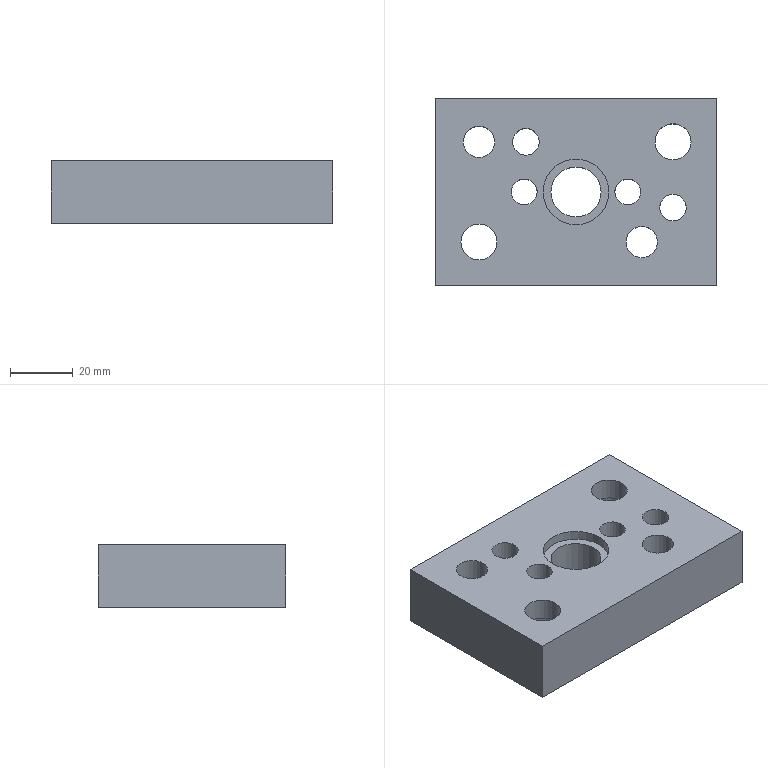Part | STEP file | lll_id3314_x_t | 1 solid | 21 faces | box 90 x 60 x 20 mm | volume 87938 mm3 | cylinder 12 | plane 9 | commonest cylinder face diameters 8.2 x2 8.505 x2 10 x2 11.509 x2 18.007 x2 16 x1
STEP:
#1=CARTESIAN_POINT('',(1798.,-16.,2.5));
#2=VERTEX_POINT('',#1);
#3=CARTESIAN_POINT('',(1803.,-16.,2.5));
#4=DIRECTION('',(0.,0.,-1.));
#5=DIRECTION('',(-1.,0.,0.));
#6=AXIS2_PLACEMENT_3D('',#3,#4,#5);
#7=CIRCLE('',#6,5.);
#8=EDGE_CURVE('',#2,#2,#7,.T.);
#9=ORIENTED_EDGE('',*,*,#8,.F.);
#10=EDGE_LOOP('',(#9));
#11=FACE_BOUND('',#10,.T.);
#12=CARTESIAN_POINT('',(1746.,16.,2.5));
#13=VERTEX_POINT('',#12);
#14=CARTESIAN_POINT('',(1751.,16.,2.5));
#15=DIRECTION('',(0.,0.,-1.));
#16=DIRECTION('',(-1.,0.,0.));
#17=AXIS2_PLACEMENT_3D('',#14,#15,#16);
#18=CIRCLE('',#17,5.);
#19=EDGE_CURVE('',#13,#13,#18,.T.);
#20=ORIENTED_EDGE('',*,*,#19,.F.);
#21=EDGE_LOOP('',(#20));
#22=FACE_BOUND('',#21,.T.);
#23=CARTESIAN_POINT('',(1813.,-9.253,2.5));
#24=VERTEX_POINT('',#23);
#25=CARTESIAN_POINT('',(1813.,-5.,2.5));
#26=DIRECTION('',(0.,0.,1.));
#27=DIRECTION('',(0.,-1.,0.));
#28=AXIS2_PLACEMENT_3D('',#25,#26,#27);
#29=CIRCLE('',#28,4.253);
#30=EDGE_CURVE('',#24,#24,#29,.T.);
#31=ORIENTED_EDGE('',*,*,#30,.T.);
#32=EDGE_LOOP('',(#31));
#33=FACE_BOUND('',#32,.T.);
#34=CARTESIAN_POINT('',(1741.996,-16.,2.5));
#35=VERTEX_POINT('',#34);
#36=CARTESIAN_POINT('',(1751.,-16.,2.5));
#37=DIRECTION('',(0.,0.,1.));
#38=DIRECTION('',(-1.,0.,0.));
#39=AXIS2_PLACEMENT_3D('',#36,#37,#38);
#40=CIRCLE('',#39,9.004);
#41=EDGE_CURVE('',#35,#35,#40,.T.);
#42=ORIENTED_EDGE('',*,*,#41,.T.);
#43=EDGE_LOOP('',(#42));
#44=FACE_BOUND('',#43,.T.);
#45=CARTESIAN_POINT('',(1827.,-30.,2.5));
#46=VERTEX_POINT('',#45);
#47=CARTESIAN_POINT('',(1827.,30.,2.5));
#48=VERTEX_POINT('',#47);
#49=CARTESIAN_POINT('',(1827.,0.,2.5));
#50=DIRECTION('',(0.,1.,0.));
#51=VECTOR('',#50,1.);
#52=LINE('',#49,#51);
#53=EDGE_CURVE('',#46,#48,#52,.T.);
#54=ORIENTED_EDGE('',*,*,#53,.F.);
#55=CARTESIAN_POINT('',(1737.,-30.,2.5));
#56=VERTEX_POINT('',#55);
#57=CARTESIAN_POINT('',(1782.,-30.,2.5));
#58=DIRECTION('',(1.,0.,0.));
#59=VECTOR('',#58,1.);
#60=LINE('',#57,#59);
#61=EDGE_CURVE('',#56,#46,#60,.T.);
#62=ORIENTED_EDGE('',*,*,#61,.F.);
#63=CARTESIAN_POINT('',(1737.,30.,2.5));
#64=VERTEX_POINT('',#63);
#65=CARTESIAN_POINT('',(1737.,0.,2.5));
#66=DIRECTION('',(0.,-1.,0.));
#67=VECTOR('',#66,1.);
#68=LINE('',#65,#67);
#69=EDGE_CURVE('',#64,#56,#68,.T.);
#70=ORIENTED_EDGE('',*,*,#69,.F.);
#71=CARTESIAN_POINT('',(1782.,30.,2.5));
#72=DIRECTION('',(-1.,0.,0.));
#73=VECTOR('',#72,1.);
#74=LINE('',#71,#73);
#75=EDGE_CURVE('',#48,#64,#74,.T.);
#76=ORIENTED_EDGE('',*,*,#75,.F.);
#77=EDGE_LOOP('',(#54,#62,#70,#76));
#78=FACE_BOUND('',#77,.T.);
#79=CARTESIAN_POINT('',(1803.997,16.,2.5));
#80=VERTEX_POINT('',#79);
#81=CARTESIAN_POINT('',(1813.,16.,2.5));
#82=DIRECTION('',(0.,0.,1.));
#83=DIRECTION('',(-1.,0.,0.));
#84=AXIS2_PLACEMENT_3D('',#81,#82,#83);
#85=CIRCLE('',#84,9.004);
#86=EDGE_CURVE('',#80,#80,#85,.T.);
#87=ORIENTED_EDGE('',*,*,#86,.T.);
#88=EDGE_LOOP('',(#87));
#89=FACE_BOUND('',#88,.T.);
#90=CARTESIAN_POINT('',(1761.4,0.,2.5));
#91=VERTEX_POINT('',#90);
#92=CARTESIAN_POINT('',(1765.5,0.,2.5));
#93=DIRECTION('',(0.,0.,-1.));
#94=DIRECTION('',(-1.,0.,0.));
#95=AXIS2_PLACEMENT_3D('',#92,#93,#94);
#96=CIRCLE('',#95,4.1);
#97=EDGE_CURVE('',#91,#91,#96,.T.);
#98=ORIENTED_EDGE('',*,*,#97,.F.);
#99=EDGE_LOOP('',(#98));
#100=FACE_BOUND('',#99,.T.);
#101=CARTESIAN_POINT('',(1794.4,0.,2.5));
#102=VERTEX_POINT('',#101);
#103=CARTESIAN_POINT('',(1798.5,0.,2.5));
#104=DIRECTION('',(0.,0.,-1.));
#105=DIRECTION('',(-1.,0.,0.));
#106=AXIS2_PLACEMENT_3D('',#103,#104,#105);
#107=CIRCLE('',#106,4.1);
#108=EDGE_CURVE('',#102,#102,#107,.T.);
#109=ORIENTED_EDGE('',*,*,#108,.F.);
#110=EDGE_LOOP('',(#109));
#111=FACE_BOUND('',#110,.T.);
#112=CARTESIAN_POINT('',(1790.,0.,2.5));
#113=VERTEX_POINT('',#112);
#114=CARTESIAN_POINT('',(1782.,0.,2.5));
#115=DIRECTION('',(0.,0.,1.));
#116=DIRECTION('',(1.,0.,0.));
#117=AXIS2_PLACEMENT_3D('',#114,#115,#116);
#118=CIRCLE('',#117,8.);
#119=EDGE_CURVE('',#113,#113,#118,.T.);
#120=ORIENTED_EDGE('',*,*,#119,.T.);
#121=EDGE_LOOP('',(#120));
#122=FACE_BOUND('',#121,.T.);
#123=CARTESIAN_POINT('',(1766.,11.747,2.5));
#124=VERTEX_POINT('',#123);
#125=CARTESIAN_POINT('',(1766.,16.,2.5));
#126=DIRECTION('',(0.,0.,1.));
#127=DIRECTION('',(0.,-1.,0.));
#128=AXIS2_PLACEMENT_3D('',#125,#126,#127);
#129=CIRCLE('',#128,4.253);
#130=EDGE_CURVE('',#124,#124,#129,.T.);
#131=ORIENTED_EDGE('',*,*,#130,.T.);
#132=EDGE_LOOP('',(#131));
#133=FACE_BOUND('',#132,.T.);
#134=CARTESIAN_POINT('',(1782.,0.,2.5));
#135=DIRECTION('',(0.,0.,-1.));
#136=DIRECTION('',(-1.,0.,0.));
#137=AXIS2_PLACEMENT_3D('',#134,#135,#136);
#138=PLANE('',#137);
#139=ADVANCED_FACE('',(#11,#22,#33,#44,#78,#89,#100,#111,#122,#133),#138,.T.);
#140=CARTESIAN_POINT('',(1766.,11.747,22.5));
#141=VERTEX_POINT('',#140);
#142=CARTESIAN_POINT('',(1766.,16.,22.5));
#143=DIRECTION('',(0.,0.,1.));
#144=DIRECTION('',(0.,-1.,0.));
#145=AXIS2_PLACEMENT_3D('',#142,#143,#144);
#146=CIRCLE('',#145,4.253);
#147=EDGE_CURVE('',#141,#141,#146,.T.);
#148=ORIENTED_EDGE('',*,*,#147,.F.);
#149=EDGE_LOOP('',(#148));
#150=FACE_BOUND('',#149,.T.);
#151=CARTESIAN_POINT('',(1813.,-9.253,22.5));
#152=VERTEX_POINT('',#151);
#153=CARTESIAN_POINT('',(1813.,-5.,22.5));
#154=DIRECTION('',(0.,0.,1.));
#155=DIRECTION('',(0.,-1.,0.));
#156=AXIS2_PLACEMENT_3D('',#153,#154,#155);
#157=CIRCLE('',#156,4.253);
#158=EDGE_CURVE('',#152,#152,#157,.T.);
#159=ORIENTED_EDGE('',*,*,#158,.F.);
#160=EDGE_LOOP('',(#159));
#161=FACE_BOUND('',#160,.T.);
#162=CARTESIAN_POINT('',(1771.5,0.,22.5));
#163=VERTEX_POINT('',#162);
#164=CARTESIAN_POINT('',(1782.,0.,22.5));
#165=DIRECTION('',(0.,0.,1.));
#166=DIRECTION('',(-1.,0.,0.));
#167=AXIS2_PLACEMENT_3D('',#164,#165,#166);
#168=CIRCLE('',#167,10.5);
#169=EDGE_CURVE('',#163,#163,#168,.T.);
#170=ORIENTED_EDGE('',*,*,#169,.F.);
#171=EDGE_LOOP('',(#170));
#172=FACE_BOUND('',#171,.T.);
#173=CARTESIAN_POINT('',(1802.6,0.,22.5));
#174=VERTEX_POINT('',#173);
#175=CARTESIAN_POINT('',(1798.5,0.,22.5));
#176=DIRECTION('',(0.,0.,1.));
#177=DIRECTION('',(1.,0.,0.));
#178=AXIS2_PLACEMENT_3D('',#175,#176,#177);
#179=CIRCLE('',#178,4.1);
#180=EDGE_CURVE('',#174,#174,#179,.T.);
#181=ORIENTED_EDGE('',*,*,#180,.F.);
#182=EDGE_LOOP('',(#181));
#183=FACE_BOUND('',#182,.T.);
#184=CARTESIAN_POINT('',(1769.6,0.,22.5));
#185=VERTEX_POINT('',#184);
#186=CARTESIAN_POINT('',(1765.5,0.,22.5));
#187=DIRECTION('',(0.,0.,1.));
#188=DIRECTION('',(1.,0.,0.));
#189=AXIS2_PLACEMENT_3D('',#186,#187,#188);
#190=CIRCLE('',#189,4.1);
#191=EDGE_CURVE('',#185,#185,#190,.T.);
#192=ORIENTED_EDGE('',*,*,#191,.F.);
#193=EDGE_LOOP('',(#192));
#194=FACE_BOUND('',#193,.T.);
#195=CARTESIAN_POINT('',(1746.,16.,22.5));
#196=VERTEX_POINT('',#195);
#197=CARTESIAN_POINT('',(1751.,16.,22.5));
#198=DIRECTION('',(0.,0.,1.));
#199=DIRECTION('',(-1.,0.,0.));
#200=AXIS2_PLACEMENT_3D('',#197,#198,#199);
#201=CIRCLE('',#200,5.);
#202=EDGE_CURVE('',#196,#196,#201,.T.);
#203=ORIENTED_EDGE('',*,*,#202,.F.);
#204=EDGE_LOOP('',(#203));
#205=FACE_BOUND('',#204,.T.);
#206=CARTESIAN_POINT('',(1745.245,-16.,22.5));
#207=VERTEX_POINT('',#206);
#208=CARTESIAN_POINT('',(1751.,-16.,22.5));
#209=DIRECTION('',(0.,0.,1.));
#210=DIRECTION('',(-1.,0.,0.));
#211=AXIS2_PLACEMENT_3D('',#208,#209,#210);
#212=CIRCLE('',#211,5.755);
#213=EDGE_CURVE('',#207,#207,#212,.T.);
#214=ORIENTED_EDGE('',*,*,#213,.F.);
#215=EDGE_LOOP('',(#214));
#216=FACE_BOUND('',#215,.T.);
#217=CARTESIAN_POINT('',(1798.,-16.,22.5));
#218=VERTEX_POINT('',#217);
#219=CARTESIAN_POINT('',(1803.,-16.,22.5));
#220=DIRECTION('',(0.,0.,1.));
#221=DIRECTION('',(-1.,0.,0.));
#222=AXIS2_PLACEMENT_3D('',#219,#220,#221);
#223=CIRCLE('',#222,5.);
#224=EDGE_CURVE('',#218,#218,#223,.T.);
#225=ORIENTED_EDGE('',*,*,#224,.F.);
#226=EDGE_LOOP('',(#225));
#227=FACE_BOUND('',#226,.T.);
#228=CARTESIAN_POINT('',(1807.246,16.,22.5));
#229=VERTEX_POINT('',#228);
#230=CARTESIAN_POINT('',(1813.,16.,22.5));
#231=DIRECTION('',(0.,0.,1.));
#232=DIRECTION('',(-1.,0.,0.));
#233=AXIS2_PLACEMENT_3D('',#230,#231,#232);
#234=CIRCLE('',#233,5.755);
#235=EDGE_CURVE('',#229,#229,#234,.T.);
#236=ORIENTED_EDGE('',*,*,#235,.F.);
#237=EDGE_LOOP('',(#236));
#238=FACE_BOUND('',#237,.T.);
#239=CARTESIAN_POINT('',(1827.,-30.,22.5));
#240=VERTEX_POINT('',#239);
#241=CARTESIAN_POINT('',(1737.,-30.,22.5));
#242=VERTEX_POINT('',#241);
#243=CARTESIAN_POINT('',(1782.,-30.,22.5));
#244=DIRECTION('',(-1.,0.,0.));
#245=VECTOR('',#244,1.);
#246=LINE('',#243,#245);
#247=EDGE_CURVE('',#240,#242,#246,.T.);
#248=ORIENTED_EDGE('',*,*,#247,.F.);
#249=CARTESIAN_POINT('',(1827.,30.,22.5));
#250=VERTEX_POINT('',#249);
#251=CARTESIAN_POINT('',(1827.,0.,22.5));
#252=DIRECTION('',(0.,-1.,0.));
#253=VECTOR('',#252,1.);
#254=LINE('',#251,#253);
#255=EDGE_CURVE('',#250,#240,#254,.T.);
#256=ORIENTED_EDGE('',*,*,#255,.F.);
#257=CARTESIAN_POINT('',(1737.,30.,22.5));
#258=VERTEX_POINT('',#257);
#259=CARTESIAN_POINT('',(1782.,30.,22.5));
#260=DIRECTION('',(1.,0.,0.));
#261=VECTOR('',#260,1.);
#262=LINE('',#259,#261);
#263=EDGE_CURVE('',#258,#250,#262,.T.);
#264=ORIENTED_EDGE('',*,*,#263,.F.);
#265=CARTESIAN_POINT('',(1737.,0.,22.5));
#266=DIRECTION('',(0.,1.,0.));
#267=VECTOR('',#266,1.);
#268=LINE('',#265,#267);
#269=EDGE_CURVE('',#242,#258,#268,.T.);
#270=ORIENTED_EDGE('',*,*,#269,.F.);
#271=EDGE_LOOP('',(#248,#256,#264,#270));
#272=FACE_BOUND('',#271,.T.);
#273=CARTESIAN_POINT('',(1782.,0.,22.5));
#274=DIRECTION('',(0.,0.,1.));
#275=DIRECTION('',(1.,0.,0.));
#276=AXIS2_PLACEMENT_3D('',#273,#274,#275);
#277=PLANE('',#276);
#278=ADVANCED_FACE('',(#150,#161,#172,#183,#194,#205,#216,#227,#238,#272),#277,.T.);
#279=CARTESIAN_POINT('',(1827.,-30.,2.5));
#280=DIRECTION('',(0.,0.,1.));
#281=VECTOR('',#280,1.);
#282=LINE('',#279,#281);
#283=EDGE_CURVE('',#46,#240,#282,.T.);
#284=ORIENTED_EDGE('',*,*,#283,.T.);
#285=ORIENTED_EDGE('',*,*,#247,.T.);
#286=CARTESIAN_POINT('',(1737.,-30.,2.5));
#287=DIRECTION('',(0.,0.,1.));
#288=VECTOR('',#287,1.);
#289=LINE('',#286,#288);
#290=EDGE_CURVE('',#56,#242,#289,.T.);
#291=ORIENTED_EDGE('',*,*,#290,.F.);
#292=ORIENTED_EDGE('',*,*,#61,.T.);
#293=EDGE_LOOP('',(#284,#285,#291,#292));
#294=FACE_OUTER_BOUND('',#293,.T.);
#295=CARTESIAN_POINT('',(1782.,-30.,2.5));
#296=DIRECTION('',(0.,-1.,0.));
#297=DIRECTION('',(0.,0.,-1.));
#298=AXIS2_PLACEMENT_3D('',#295,#296,#297);
#299=PLANE('',#298);
#300=ADVANCED_FACE('',(#294),#299,.T.);
#301=ORIENTED_EDGE('',*,*,#290,.T.);
#302=ORIENTED_EDGE('',*,*,#269,.T.);
#303=CARTESIAN_POINT('',(1737.,30.,2.5));
#304=DIRECTION('',(0.,0.,1.));
#305=VECTOR('',#304,1.);
#306=LINE('',#303,#305);
#307=EDGE_CURVE('',#64,#258,#306,.T.);
#308=ORIENTED_EDGE('',*,*,#307,.F.);
#309=ORIENTED_EDGE('',*,*,#69,.T.);
#310=EDGE_LOOP('',(#301,#302,#308,#309));
#311=FACE_OUTER_BOUND('',#310,.T.);
#312=CARTESIAN_POINT('',(1737.,0.,2.5));
#313=DIRECTION('',(-1.,0.,0.));
#314=DIRECTION('',(0.,0.,1.));
#315=AXIS2_PLACEMENT_3D('',#312,#313,#314);
#316=PLANE('',#315);
#317=ADVANCED_FACE('',(#311),#316,.T.);
#318=ORIENTED_EDGE('',*,*,#307,.T.);
#319=ORIENTED_EDGE('',*,*,#263,.T.);
#320=CARTESIAN_POINT('',(1827.,30.,2.5));
#321=DIRECTION('',(0.,0.,1.));
#322=VECTOR('',#321,1.);
#323=LINE('',#320,#322);
#324=EDGE_CURVE('',#48,#250,#323,.T.);
#325=ORIENTED_EDGE('',*,*,#324,.F.);
#326=ORIENTED_EDGE('',*,*,#75,.T.);
#327=EDGE_LOOP('',(#318,#319,#325,#326));
#328=FACE_OUTER_BOUND('',#327,.T.);
#329=CARTESIAN_POINT('',(1782.,30.,2.5));
#330=DIRECTION('',(0.,1.,0.));
#331=DIRECTION('',(0.,0.,1.));
#332=AXIS2_PLACEMENT_3D('',#329,#330,#331);
#333=PLANE('',#332);
#334=ADVANCED_FACE('',(#328),#333,.T.);
#335=ORIENTED_EDGE('',*,*,#53,.T.);
#336=ORIENTED_EDGE('',*,*,#324,.T.);
#337=ORIENTED_EDGE('',*,*,#255,.T.);
#338=ORIENTED_EDGE('',*,*,#283,.F.);
#339=EDGE_LOOP('',(#335,#336,#337,#338));
#340=FACE_OUTER_BOUND('',#339,.T.);
#341=CARTESIAN_POINT('',(1827.,0.,2.5));
#342=DIRECTION('',(1.,0.,0.));
#343=DIRECTION('',(0.,0.,-1.));
#344=AXIS2_PLACEMENT_3D('',#341,#342,#343);
#345=PLANE('',#344);
#346=ADVANCED_FACE('',(#340),#345,.T.);
#347=ORIENTED_EDGE('',*,*,#235,.T.);
#348=EDGE_LOOP('',(#347));
#349=FACE_BOUND('',#348,.T.);
#350=CARTESIAN_POINT('',(1807.246,16.,15.5));
#351=VERTEX_POINT('',#350);
#352=CARTESIAN_POINT('',(1813.,16.,15.5));
#353=DIRECTION('',(0.,0.,1.));
#354=DIRECTION('',(-1.,0.,0.));
#355=AXIS2_PLACEMENT_3D('',#352,#353,#354);
#356=CIRCLE('',#355,5.755);
#357=EDGE_CURVE('',#351,#351,#356,.T.);
#358=ORIENTED_EDGE('',*,*,#357,.F.);
#359=EDGE_LOOP('',(#358));
#360=FACE_BOUND('',#359,.T.);
#361=CARTESIAN_POINT('',(1813.,16.,-2.5));
#362=DIRECTION('',(0.,0.,1.));
#363=DIRECTION('',(-1.,0.,0.));
#364=AXIS2_PLACEMENT_3D('',#361,#362,#363);
#365=CYLINDRICAL_SURFACE('',#364,5.755);
#366=ADVANCED_FACE('',(#349,#360),#365,.F.);
#367=ORIENTED_EDGE('',*,*,#357,.T.);
#368=EDGE_LOOP('',(#367));
#369=FACE_BOUND('',#368,.T.);
#370=CARTESIAN_POINT('',(1803.997,16.,15.5));
#371=VERTEX_POINT('',#370);
#372=CARTESIAN_POINT('',(1813.,16.,15.5));
#373=DIRECTION('',(0.,0.,1.));
#374=DIRECTION('',(-1.,0.,0.));
#375=AXIS2_PLACEMENT_3D('',#372,#373,#374);
#376=CIRCLE('',#375,9.004);
#377=EDGE_CURVE('',#371,#371,#376,.T.);
#378=ORIENTED_EDGE('',*,*,#377,.F.);
#379=EDGE_LOOP('',(#378));
#380=FACE_BOUND('',#379,.T.);
#381=CARTESIAN_POINT('',(1813.,16.,15.5));
#382=DIRECTION('',(0.,0.,1.));
#383=DIRECTION('',(-1.,0.,0.));
#384=AXIS2_PLACEMENT_3D('',#381,#382,#383);
#385=PLANE('',#384);
#386=ADVANCED_FACE('',(#369,#380),#385,.F.);
#387=ORIENTED_EDGE('',*,*,#377,.T.);
#388=EDGE_LOOP('',(#387));
#389=FACE_BOUND('',#388,.T.);
#390=ORIENTED_EDGE('',*,*,#86,.F.);
#391=EDGE_LOOP('',(#390));
#392=FACE_BOUND('',#391,.T.);
#393=CARTESIAN_POINT('',(1813.,16.,2.5));
#394=DIRECTION('',(0.,0.,1.));
#395=DIRECTION('',(-1.,0.,0.));
#396=AXIS2_PLACEMENT_3D('',#393,#394,#395);
#397=CYLINDRICAL_SURFACE('',#396,9.004);
#398=ADVANCED_FACE('',(#389,#392),#397,.F.);
#399=ORIENTED_EDGE('',*,*,#224,.T.);
#400=EDGE_LOOP('',(#399));
#401=FACE_BOUND('',#400,.T.);
#402=ORIENTED_EDGE('',*,*,#8,.T.);
#403=EDGE_LOOP('',(#402));
#404=FACE_BOUND('',#403,.T.);
#405=CARTESIAN_POINT('',(1803.,-16.,-2.5));
#406=DIRECTION('',(0.,0.,1.));
#407=DIRECTION('',(-1.,0.,0.));
#408=AXIS2_PLACEMENT_3D('',#405,#406,#407);
#409=CYLINDRICAL_SURFACE('',#408,5.);
#410=ADVANCED_FACE('',(#401,#404),#409,.F.);
#411=ORIENTED_EDGE('',*,*,#213,.T.);
#412=EDGE_LOOP('',(#411));
#413=FACE_BOUND('',#412,.T.);
#414=CARTESIAN_POINT('',(1745.245,-16.,15.5));
#415=VERTEX_POINT('',#414);
#416=CARTESIAN_POINT('',(1751.,-16.,15.5));
#417=DIRECTION('',(0.,0.,1.));
#418=DIRECTION('',(-1.,0.,0.));
#419=AXIS2_PLACEMENT_3D('',#416,#417,#418);
#420=CIRCLE('',#419,5.755);
#421=EDGE_CURVE('',#415,#415,#420,.T.);
#422=ORIENTED_EDGE('',*,*,#421,.F.);
#423=EDGE_LOOP('',(#422));
#424=FACE_BOUND('',#423,.T.);
#425=CARTESIAN_POINT('',(1751.,-16.,-2.5));
#426=DIRECTION('',(0.,0.,1.));
#427=DIRECTION('',(-1.,0.,0.));
#428=AXIS2_PLACEMENT_3D('',#425,#426,#427);
#429=CYLINDRICAL_SURFACE('',#428,5.755);
#430=ADVANCED_FACE('',(#413,#424),#429,.F.);
#431=ORIENTED_EDGE('',*,*,#421,.T.);
#432=EDGE_LOOP('',(#431));
#433=FACE_BOUND('',#432,.T.);
#434=CARTESIAN_POINT('',(1741.996,-16.,15.5));
#435=VERTEX_POINT('',#434);
#436=CARTESIAN_POINT('',(1751.,-16.,15.5));
#437=DIRECTION('',(0.,0.,1.));
#438=DIRECTION('',(-1.,0.,0.));
#439=AXIS2_PLACEMENT_3D('',#436,#437,#438);
#440=CIRCLE('',#439,9.004);
#441=EDGE_CURVE('',#435,#435,#440,.T.);
#442=ORIENTED_EDGE('',*,*,#441,.F.);
#443=EDGE_LOOP('',(#442));
#444=FACE_BOUND('',#443,.T.);
#445=CARTESIAN_POINT('',(1751.,-16.,15.5));
#446=DIRECTION('',(0.,0.,1.));
#447=DIRECTION('',(-1.,0.,0.));
#448=AXIS2_PLACEMENT_3D('',#445,#446,#447);
#449=PLANE('',#448);
#450=ADVANCED_FACE('',(#433,#444),#449,.F.);
#451=ORIENTED_EDGE('',*,*,#441,.T.);
#452=EDGE_LOOP('',(#451));
#453=FACE_BOUND('',#452,.T.);
#454=ORIENTED_EDGE('',*,*,#41,.F.);
#455=EDGE_LOOP('',(#454));
#456=FACE_BOUND('',#455,.T.);
#457=CARTESIAN_POINT('',(1751.,-16.,2.5));
#458=DIRECTION('',(0.,0.,1.));
#459=DIRECTION('',(-1.,0.,0.));
#460=AXIS2_PLACEMENT_3D('',#457,#458,#459);
#461=CYLINDRICAL_SURFACE('',#460,9.004);
#462=ADVANCED_FACE('',(#453,#456),#461,.F.);
#463=ORIENTED_EDGE('',*,*,#202,.T.);
#464=EDGE_LOOP('',(#463));
#465=FACE_BOUND('',#464,.T.);
#466=ORIENTED_EDGE('',*,*,#19,.T.);
#467=EDGE_LOOP('',(#466));
#468=FACE_BOUND('',#467,.T.);
#469=CARTESIAN_POINT('',(1751.,16.,-2.5));
#470=DIRECTION('',(0.,0.,1.));
#471=DIRECTION('',(-1.,0.,0.));
#472=AXIS2_PLACEMENT_3D('',#469,#470,#471);
#473=CYLINDRICAL_SURFACE('',#472,5.);
#474=ADVANCED_FACE('',(#465,#468),#473,.F.);
#475=ORIENTED_EDGE('',*,*,#97,.T.);
#476=EDGE_LOOP('',(#475));
#477=FACE_BOUND('',#476,.T.);
#478=ORIENTED_EDGE('',*,*,#191,.T.);
#479=EDGE_LOOP('',(#478));
#480=FACE_BOUND('',#479,.T.);
#481=CARTESIAN_POINT('',(1765.5,0.,-2.5));
#482=DIRECTION('',(0.,0.,1.));
#483=DIRECTION('',(1.,0.,0.));
#484=AXIS2_PLACEMENT_3D('',#481,#482,#483);
#485=CYLINDRICAL_SURFACE('',#484,4.1);
#486=ADVANCED_FACE('',(#477,#480),#485,.F.);
#487=ORIENTED_EDGE('',*,*,#108,.T.);
#488=EDGE_LOOP('',(#487));
#489=FACE_BOUND('',#488,.T.);
#490=ORIENTED_EDGE('',*,*,#180,.T.);
#491=EDGE_LOOP('',(#490));
#492=FACE_BOUND('',#491,.T.);
#493=CARTESIAN_POINT('',(1798.5,0.,-2.5));
#494=DIRECTION('',(0.,0.,1.));
#495=DIRECTION('',(1.,0.,0.));
#496=AXIS2_PLACEMENT_3D('',#493,#494,#495);
#497=CYLINDRICAL_SURFACE('',#496,4.1);
#498=ADVANCED_FACE('',(#489,#492),#497,.F.);
#499=CARTESIAN_POINT('',(1771.5,0.,19.5));
#500=VERTEX_POINT('',#499);
#501=CARTESIAN_POINT('',(1782.,0.,19.5));
#502=DIRECTION('',(0.,0.,1.));
#503=DIRECTION('',(-1.,0.,0.));
#504=AXIS2_PLACEMENT_3D('',#501,#502,#503);
#505=CIRCLE('',#504,10.5);
#506=EDGE_CURVE('',#500,#500,#505,.T.);
#507=ORIENTED_EDGE('',*,*,#506,.T.);
#508=EDGE_LOOP('',(#507));
#509=FACE_BOUND('',#508,.T.);
#510=CARTESIAN_POINT('',(1774.,0.,19.5));
#511=VERTEX_POINT('',#510);
#512=CARTESIAN_POINT('',(1782.,0.,19.5));
#513=DIRECTION('',(0.,0.,-1.));
#514=DIRECTION('',(-1.,0.,0.));
#515=AXIS2_PLACEMENT_3D('',#512,#513,#514);
#516=CIRCLE('',#515,8.);
#517=EDGE_CURVE('',#511,#511,#516,.T.);
#518=ORIENTED_EDGE('',*,*,#517,.T.);
#519=EDGE_LOOP('',(#518));
#520=FACE_BOUND('',#519,.T.);
#521=CARTESIAN_POINT('',(1782.,0.,19.5));
#522=DIRECTION('',(0.,0.,-1.));
#523=DIRECTION('',(0.,-1.,0.));
#524=AXIS2_PLACEMENT_3D('',#521,#522,#523);
#525=PLANE('',#524);
#526=ADVANCED_FACE('',(#509,#520),#525,.F.);
#527=ORIENTED_EDGE('',*,*,#169,.T.);
#528=EDGE_LOOP('',(#527));
#529=FACE_BOUND('',#528,.T.);
#530=ORIENTED_EDGE('',*,*,#506,.F.);
#531=EDGE_LOOP('',(#530));
#532=FACE_BOUND('',#531,.T.);
#533=CARTESIAN_POINT('',(1782.,0.,19.5));
#534=DIRECTION('',(0.,0.,-1.));
#535=DIRECTION('',(0.,-1.,0.));
#536=AXIS2_PLACEMENT_3D('',#533,#534,#535);
#537=CYLINDRICAL_SURFACE('',#536,10.5);
#538=ADVANCED_FACE('',(#529,#532),#537,.F.);
#539=ORIENTED_EDGE('',*,*,#119,.F.);
#540=EDGE_LOOP('',(#539));
#541=FACE_BOUND('',#540,.T.);
#542=ORIENTED_EDGE('',*,*,#517,.F.);
#543=EDGE_LOOP('',(#542));
#544=FACE_BOUND('',#543,.T.);
#545=CARTESIAN_POINT('',(1782.,0.,20.5));
#546=DIRECTION('',(0.,0.,-1.));
#547=DIRECTION('',(0.,-1.,0.));
#548=AXIS2_PLACEMENT_3D('',#545,#546,#547);
#549=CYLINDRICAL_SURFACE('',#548,8.);
#550=ADVANCED_FACE('',(#541,#544),#549,.F.);
#551=ORIENTED_EDGE('',*,*,#158,.T.);
#552=EDGE_LOOP('',(#551));
#553=FACE_BOUND('',#552,.T.);
#554=ORIENTED_EDGE('',*,*,#30,.F.);
#555=EDGE_LOOP('',(#554));
#556=FACE_BOUND('',#555,.T.);
#557=CARTESIAN_POINT('',(1813.,-5.,2.5));
#558=DIRECTION('',(0.,0.,1.));
#559=DIRECTION('',(0.,-1.,0.));
#560=AXIS2_PLACEMENT_3D('',#557,#558,#559);
#561=CYLINDRICAL_SURFACE('',#560,4.253);
#562=ADVANCED_FACE('',(#553,#556),#561,.F.);
#563=ORIENTED_EDGE('',*,*,#147,.T.);
#564=EDGE_LOOP('',(#563));
#565=FACE_BOUND('',#564,.T.);
#566=ORIENTED_EDGE('',*,*,#130,.F.);
#567=EDGE_LOOP('',(#566));
#568=FACE_BOUND('',#567,.T.);
#569=CARTESIAN_POINT('',(1766.,16.,2.5));
#570=DIRECTION('',(0.,0.,1.));
#571=DIRECTION('',(0.,-1.,0.));
#572=AXIS2_PLACEMENT_3D('',#569,#570,#571);
#573=CYLINDRICAL_SURFACE('',#572,4.253);
#574=ADVANCED_FACE('',(#565,#568),#573,.F.);
#575=CLOSED_SHELL('',(#139,#278,#300,#317,#334,#346,#366,#386,#398,#410,#430,#450,#462,#474,#486,#498,#526,#538,#550,#562,#574));
#576=MANIFOLD_SOLID_BREP('',#575);
#577=(LENGTH_UNIT()NAMED_UNIT(*)SI_UNIT(.MILLI.,.METRE.));
#578=UNCERTAINTY_MEASURE_WITH_UNIT(LENGTH_MEASURE(0.00002),#577,'','');
#579=(NAMED_UNIT(*)PLANE_ANGLE_UNIT()SI_UNIT($,.RADIAN.));
#580=PLANE_ANGLE_MEASURE_WITH_UNIT(PLANE_ANGLE_MEASURE(0.01745),#579);
#581=DIMENSIONAL_EXPONENTS(0.,0.,0.,0.,0.,0.,0.);
#582=(CONVERSION_BASED_UNIT('DEGREE',#580)NAMED_UNIT(#581)PLANE_ANGLE_UNIT());
#583=(NAMED_UNIT(*)SI_UNIT($,.STERADIAN.)SOLID_ANGLE_UNIT());
#584=(GEOMETRIC_REPRESENTATION_CONTEXT(3)GLOBAL_UNCERTAINTY_ASSIGNED_CONTEXT((#578))GLOBAL_UNIT_ASSIGNED_CONTEXT((#577,#582,#583))REPRESENTATION_CONTEXT('',''));
#585=ADVANCED_BREP_SHAPE_REPRESENTATION('',(#576),#584);